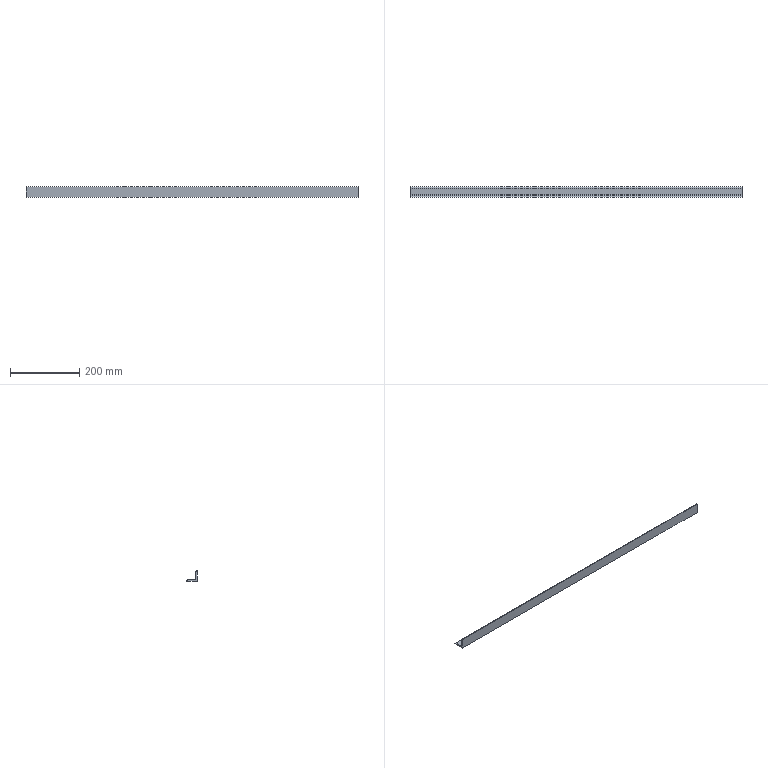Part | STEP file | Angle steel_Default<machined> | 1 solid | 9 faces | box 960 x 30 x 30 mm | volume 210971 mm3 | plane 6 | cylinder 3 | commonest cylinder face diameters 8 x2 7 x1
STEP:
#1=CARTESIAN_POINT('',(0.,0.,0.));
#2=VERTEX_POINT('',#1);
#3=CARTESIAN_POINT('',(0.,0.,30.));
#4=VERTEX_POINT('',#3);
#5=CARTESIAN_POINT('',(0.,0.,30.));
#6=DIRECTION('',(0.,0.,1.));
#7=VECTOR('',#6,1000.);
#8=LINE('',#5,#7);
#9=EDGE_CURVE('',#2,#4,#8,.T.);
#10=ORIENTED_EDGE('',*,*,#9,.T.);
#11=CARTESIAN_POINT('',(-960.,0.,30.));
#12=VERTEX_POINT('',#11);
#13=CARTESIAN_POINT('',(-960.,0.,30.));
#14=DIRECTION('',(1.,0.,0.));
#15=VECTOR('',#14,1000.);
#16=LINE('',#13,#15);
#17=EDGE_CURVE('',#12,#4,#16,.T.);
#18=ORIENTED_EDGE('',*,*,#17,.F.);
#19=CARTESIAN_POINT('',(-960.,0.,0.));
#20=VERTEX_POINT('',#19);
#21=CARTESIAN_POINT('',(-960.,0.,30.));
#22=DIRECTION('',(0.,0.,1.));
#23=VECTOR('',#22,1000.);
#24=LINE('',#21,#23);
#25=EDGE_CURVE('',#20,#12,#24,.T.);
#26=ORIENTED_EDGE('',*,*,#25,.F.);
#27=CARTESIAN_POINT('',(-960.,0.,0.));
#28=DIRECTION('',(1.,0.,0.));
#29=VECTOR('',#28,1000.);
#30=LINE('',#27,#29);
#31=EDGE_CURVE('',#20,#2,#30,.T.);
#32=ORIENTED_EDGE('',*,*,#31,.T.);
#33=EDGE_LOOP('',(#10,#18,#26,#32));
#34=FACE_OUTER_BOUND('',#33,.T.);
#35=CARTESIAN_POINT('',(-960.,0.,30.));
#36=DIRECTION('',(0.,1.,0.));
#37=DIRECTION('',(0.,0.,1.));
#38=AXIS2_PLACEMENT_3D('',#35,#36,#37);
#39=PLANE('',#38);
#40=ADVANCED_FACE('',(#34),#39,.F.);
#41=CARTESIAN_POINT('',(0.,4.,26.));
#42=VERTEX_POINT('',#41);
#43=CARTESIAN_POINT('',(0.,0.,26.));
#44=DIRECTION('',(-1.,0.,0.));
#45=DIRECTION('',(0.,0.,1.));
#46=AXIS2_PLACEMENT_3D('',#43,#44,#45);
#47=CIRCLE('',#46,4.);
#48=EDGE_CURVE('',#4,#42,#47,.T.);
#49=ORIENTED_EDGE('',*,*,#48,.T.);
#50=CARTESIAN_POINT('',(-960.,4.,26.));
#51=VERTEX_POINT('',#50);
#52=CARTESIAN_POINT('',(-960.,4.,26.));
#53=DIRECTION('',(1.,0.,0.));
#54=VECTOR('',#53,1000.);
#55=LINE('',#52,#54);
#56=EDGE_CURVE('',#51,#42,#55,.T.);
#57=ORIENTED_EDGE('',*,*,#56,.F.);
#58=CARTESIAN_POINT('',(-960.,0.,26.));
#59=DIRECTION('',(-1.,0.,0.));
#60=DIRECTION('',(0.,0.,1.));
#61=AXIS2_PLACEMENT_3D('',#58,#59,#60);
#62=CIRCLE('',#61,4.);
#63=EDGE_CURVE('',#12,#51,#62,.T.);
#64=ORIENTED_EDGE('',*,*,#63,.F.);
#65=ORIENTED_EDGE('',*,*,#17,.T.);
#66=EDGE_LOOP('',(#49,#57,#64,#65));
#67=FACE_OUTER_BOUND('',#66,.T.);
#68=CARTESIAN_POINT('',(-960.,0.,26.));
#69=DIRECTION('',(1.,0.,0.));
#70=DIRECTION('',(0.,0.,-1.));
#71=AXIS2_PLACEMENT_3D('',#68,#69,#70);
#72=CYLINDRICAL_SURFACE('',#71,4.);
#73=ADVANCED_FACE('',(#67),#72,.T.);
#74=CARTESIAN_POINT('',(0.,4.,7.5));
#75=VERTEX_POINT('',#74);
#76=CARTESIAN_POINT('',(0.,4.,7.5));
#77=DIRECTION('',(0.,0.,-1.));
#78=VECTOR('',#77,1000.);
#79=LINE('',#76,#78);
#80=EDGE_CURVE('',#42,#75,#79,.T.);
#81=ORIENTED_EDGE('',*,*,#80,.T.);
#82=CARTESIAN_POINT('',(-960.,4.,7.5));
#83=VERTEX_POINT('',#82);
#84=CARTESIAN_POINT('',(-960.,4.,7.5));
#85=DIRECTION('',(1.,0.,0.));
#86=VECTOR('',#85,1000.);
#87=LINE('',#84,#86);
#88=EDGE_CURVE('',#83,#75,#87,.T.);
#89=ORIENTED_EDGE('',*,*,#88,.F.);
#90=CARTESIAN_POINT('',(-960.,4.,7.5));
#91=DIRECTION('',(0.,0.,-1.));
#92=VECTOR('',#91,1000.);
#93=LINE('',#90,#92);
#94=EDGE_CURVE('',#51,#83,#93,.T.);
#95=ORIENTED_EDGE('',*,*,#94,.F.);
#96=ORIENTED_EDGE('',*,*,#56,.T.);
#97=EDGE_LOOP('',(#81,#89,#95,#96));
#98=FACE_OUTER_BOUND('',#97,.T.);
#99=CARTESIAN_POINT('',(-960.,4.,7.5));
#100=DIRECTION('',(0.,-1.,0.));
#101=DIRECTION('',(0.,0.,-1.));
#102=AXIS2_PLACEMENT_3D('',#99,#100,#101);
#103=PLANE('',#102);
#104=ADVANCED_FACE('',(#98),#103,.F.);
#105=CARTESIAN_POINT('',(0.,7.5,4.));
#106=VERTEX_POINT('',#105);
#107=CARTESIAN_POINT('',(0.,7.5,7.5));
#108=DIRECTION('',(1.,0.,0.));
#109=DIRECTION('',(0.,0.,-1.));
#110=AXIS2_PLACEMENT_3D('',#107,#108,#109);
#111=CIRCLE('',#110,3.5);
#112=EDGE_CURVE('',#75,#106,#111,.T.);
#113=ORIENTED_EDGE('',*,*,#112,.T.);
#114=CARTESIAN_POINT('',(-960.,7.5,4.));
#115=VERTEX_POINT('',#114);
#116=CARTESIAN_POINT('',(-960.,7.5,4.));
#117=DIRECTION('',(1.,0.,0.));
#118=VECTOR('',#117,1000.);
#119=LINE('',#116,#118);
#120=EDGE_CURVE('',#115,#106,#119,.T.);
#121=ORIENTED_EDGE('',*,*,#120,.F.);
#122=CARTESIAN_POINT('',(-960.,7.5,7.5));
#123=DIRECTION('',(1.,0.,0.));
#124=DIRECTION('',(0.,0.,-1.));
#125=AXIS2_PLACEMENT_3D('',#122,#123,#124);
#126=CIRCLE('',#125,3.5);
#127=EDGE_CURVE('',#83,#115,#126,.T.);
#128=ORIENTED_EDGE('',*,*,#127,.F.);
#129=ORIENTED_EDGE('',*,*,#88,.T.);
#130=EDGE_LOOP('',(#113,#121,#128,#129));
#131=FACE_OUTER_BOUND('',#130,.T.);
#132=CARTESIAN_POINT('',(-960.,7.5,7.5));
#133=DIRECTION('',(1.,0.,0.));
#134=DIRECTION('',(0.,0.,-1.));
#135=AXIS2_PLACEMENT_3D('',#132,#133,#134);
#136=CYLINDRICAL_SURFACE('',#135,3.5);
#137=ADVANCED_FACE('',(#131),#136,.F.);
#138=CARTESIAN_POINT('',(0.,26.,4.));
#139=VERTEX_POINT('',#138);
#140=CARTESIAN_POINT('',(0.,26.,4.));
#141=DIRECTION('',(0.,1.,0.));
#142=VECTOR('',#141,1000.);
#143=LINE('',#140,#142);
#144=EDGE_CURVE('',#106,#139,#143,.T.);
#145=ORIENTED_EDGE('',*,*,#144,.T.);
#146=CARTESIAN_POINT('',(-960.,26.,4.));
#147=VERTEX_POINT('',#146);
#148=CARTESIAN_POINT('',(-960.,26.,4.));
#149=DIRECTION('',(1.,0.,0.));
#150=VECTOR('',#149,1000.);
#151=LINE('',#148,#150);
#152=EDGE_CURVE('',#147,#139,#151,.T.);
#153=ORIENTED_EDGE('',*,*,#152,.F.);
#154=CARTESIAN_POINT('',(-960.,26.,4.));
#155=DIRECTION('',(0.,1.,0.));
#156=VECTOR('',#155,1000.);
#157=LINE('',#154,#156);
#158=EDGE_CURVE('',#115,#147,#157,.T.);
#159=ORIENTED_EDGE('',*,*,#158,.F.);
#160=ORIENTED_EDGE('',*,*,#120,.T.);
#161=EDGE_LOOP('',(#145,#153,#159,#160));
#162=FACE_OUTER_BOUND('',#161,.T.);
#163=CARTESIAN_POINT('',(-960.,26.,4.));
#164=DIRECTION('',(0.,0.,-1.));
#165=DIRECTION('',(0.,1.,0.));
#166=AXIS2_PLACEMENT_3D('',#163,#164,#165);
#167=PLANE('',#166);
#168=ADVANCED_FACE('',(#162),#167,.F.);
#169=CARTESIAN_POINT('',(0.,30.,0.));
#170=VERTEX_POINT('',#169);
#171=CARTESIAN_POINT('',(0.,26.,0.));
#172=DIRECTION('',(-1.,0.,0.));
#173=DIRECTION('',(0.,0.,-1.));
#174=AXIS2_PLACEMENT_3D('',#171,#172,#173);
#175=CIRCLE('',#174,4.);
#176=EDGE_CURVE('',#139,#170,#175,.T.);
#177=ORIENTED_EDGE('',*,*,#176,.T.);
#178=CARTESIAN_POINT('',(-960.,30.,0.));
#179=VERTEX_POINT('',#178);
#180=CARTESIAN_POINT('',(-960.,30.,0.));
#181=DIRECTION('',(1.,0.,0.));
#182=VECTOR('',#181,1000.);
#183=LINE('',#180,#182);
#184=EDGE_CURVE('',#179,#170,#183,.T.);
#185=ORIENTED_EDGE('',*,*,#184,.F.);
#186=CARTESIAN_POINT('',(-960.,26.,0.));
#187=DIRECTION('',(-1.,0.,0.));
#188=DIRECTION('',(0.,0.,-1.));
#189=AXIS2_PLACEMENT_3D('',#186,#187,#188);
#190=CIRCLE('',#189,4.);
#191=EDGE_CURVE('',#147,#179,#190,.T.);
#192=ORIENTED_EDGE('',*,*,#191,.F.);
#193=ORIENTED_EDGE('',*,*,#152,.T.);
#194=EDGE_LOOP('',(#177,#185,#192,#193));
#195=FACE_OUTER_BOUND('',#194,.T.);
#196=CARTESIAN_POINT('',(-960.,26.,0.));
#197=DIRECTION('',(1.,0.,0.));
#198=DIRECTION('',(0.,0.,-1.));
#199=AXIS2_PLACEMENT_3D('',#196,#197,#198);
#200=CYLINDRICAL_SURFACE('',#199,4.);
#201=ADVANCED_FACE('',(#195),#200,.T.);
#202=CARTESIAN_POINT('',(0.,0.,0.));
#203=DIRECTION('',(0.,-1.,0.));
#204=VECTOR('',#203,1000.);
#205=LINE('',#202,#204);
#206=EDGE_CURVE('',#170,#2,#205,.T.);
#207=ORIENTED_EDGE('',*,*,#206,.T.);
#208=ORIENTED_EDGE('',*,*,#31,.F.);
#209=CARTESIAN_POINT('',(-960.,0.,0.));
#210=DIRECTION('',(0.,-1.,0.));
#211=VECTOR('',#210,1000.);
#212=LINE('',#209,#211);
#213=EDGE_CURVE('',#179,#20,#212,.T.);
#214=ORIENTED_EDGE('',*,*,#213,.F.);
#215=ORIENTED_EDGE('',*,*,#184,.T.);
#216=EDGE_LOOP('',(#207,#208,#214,#215));
#217=FACE_OUTER_BOUND('',#216,.T.);
#218=CARTESIAN_POINT('',(-960.,0.,0.));
#219=DIRECTION('',(0.,0.,1.));
#220=DIRECTION('',(1.,0.,0.));
#221=AXIS2_PLACEMENT_3D('',#218,#219,#220);
#222=PLANE('',#221);
#223=ADVANCED_FACE('',(#217),#222,.F.);
#224=ORIENTED_EDGE('',*,*,#25,.T.);
#225=ORIENTED_EDGE('',*,*,#63,.T.);
#226=ORIENTED_EDGE('',*,*,#94,.T.);
#227=ORIENTED_EDGE('',*,*,#127,.T.);
#228=ORIENTED_EDGE('',*,*,#158,.T.);
#229=ORIENTED_EDGE('',*,*,#191,.T.);
#230=ORIENTED_EDGE('',*,*,#213,.T.);
#231=EDGE_LOOP('',(#224,#225,#226,#227,#228,#229,#230));
#232=FACE_OUTER_BOUND('',#231,.T.);
#233=CARTESIAN_POINT('',(-960.,26.,0.));
#234=DIRECTION('',(1.,0.,0.));
#235=DIRECTION('',(0.,0.,-1.));
#236=AXIS2_PLACEMENT_3D('',#233,#234,#235);
#237=PLANE('',#236);
#238=ADVANCED_FACE('',(#232),#237,.F.);
#239=ORIENTED_EDGE('',*,*,#9,.F.);
#240=ORIENTED_EDGE('',*,*,#206,.F.);
#241=ORIENTED_EDGE('',*,*,#176,.F.);
#242=ORIENTED_EDGE('',*,*,#144,.F.);
#243=ORIENTED_EDGE('',*,*,#112,.F.);
#244=ORIENTED_EDGE('',*,*,#80,.F.);
#245=ORIENTED_EDGE('',*,*,#48,.F.);
#246=EDGE_LOOP('',(#239,#240,#241,#242,#243,#244,#245));
#247=FACE_OUTER_BOUND('',#246,.T.);
#248=CARTESIAN_POINT('',(0.,26.,0.));
#249=DIRECTION('',(1.,0.,0.));
#250=DIRECTION('',(0.,0.,-1.));
#251=AXIS2_PLACEMENT_3D('',#248,#249,#250);
#252=PLANE('',#251);
#253=ADVANCED_FACE('',(#247),#252,.T.);
#254=CLOSED_SHELL('',(#40,#73,#104,#137,#168,#201,#223,#238,#253));
#255=MANIFOLD_SOLID_BREP('',#254);
#256=CARTESIAN_POINT('',(0.,0.,0.));
#257=DIRECTION('',(0.,0.,1.));
#258=DIRECTION('',(1.,0.,0.));
#259=AXIS2_PLACEMENT_3D('',#256,#257,#258);
#260=(LENGTH_UNIT()NAMED_UNIT(*)SI_UNIT(.MILLI.,.METRE.));
#261=UNCERTAINTY_MEASURE_WITH_UNIT(LENGTH_MEASURE(0.00001),#260,'','');
#262=(NAMED_UNIT(*)PLANE_ANGLE_UNIT()SI_UNIT($,.RADIAN.));
#263=(NAMED_UNIT(*)SI_UNIT($,.STERADIAN.)SOLID_ANGLE_UNIT());
#264=(GEOMETRIC_REPRESENTATION_CONTEXT(3)GLOBAL_UNCERTAINTY_ASSIGNED_CONTEXT((#261))GLOBAL_UNIT_ASSIGNED_CONTEXT((#260,#262,#263))REPRESENTATION_CONTEXT('',''));
#265=ADVANCED_BREP_SHAPE_REPRESENTATION('',(#255,#259),#264);